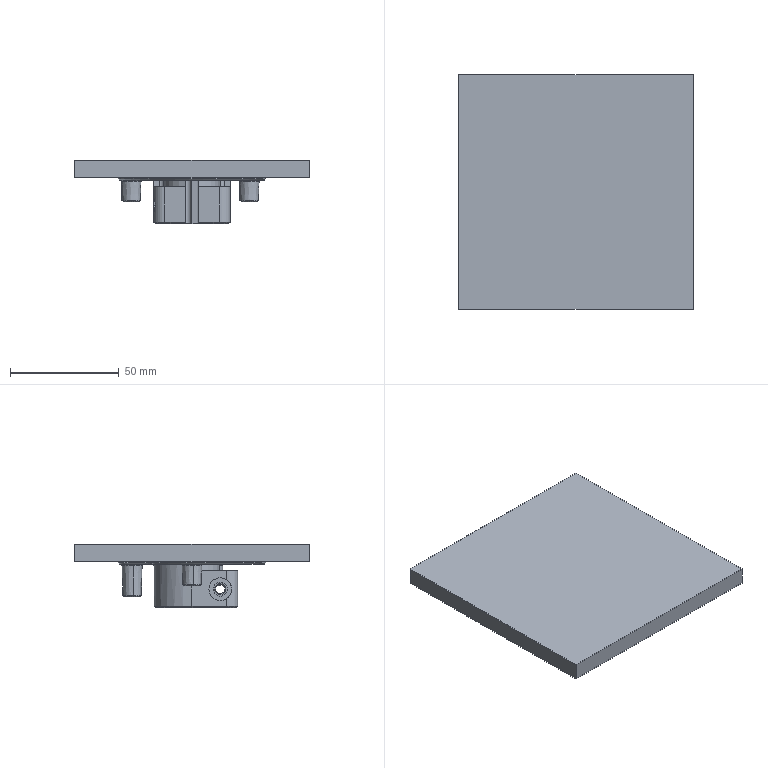NC program | NX | posted with a generic post | part box 108 x 108 x 29 mm
Lines 5648 to 6222 of 13118:
(ZLEVEL_PROFILE_COPY_COPY_COPY_1_COPY , TOOL : D4)
N11234 T15 M6
N11236 G54
N11238 G17 G0 G90 X-15.3 Y-3.944 S9500 M3
N11240 G43 Z30. H15
N11242 Z-0.4
N11244 G94 G1 X-14.797 Y-3.492 F1000.
N11246 G3 X-14.674 Y-3.112 R0.4
N11248 G2 X-14.866 Y-2. R15. F1500.
N11250 G1 X-16.015
N11252 G3 X-16.362 Y-2.2 R0.4
N11254 G1 Y-2.8
N11256 G0 X-15.3 Y-3.944 Z-0.8
N11258 G1 X-14.797 Y-3.492 F1000.
N11260 G3 X-14.674 Y-3.112 R0.4
N11262 G2 X-14.866 Y-2. R15. F1500.
N11264 G1 X-16.015
N11266 G3 X-16.362 Y-2.2 R0.4
N11268 G1 Y-2.8
N11270 G0 X-15.3 Y-3.944 Z-1.2
N11272 G1 X-14.797 Y-3.492 F1000.
N11274 G3 X-14.674 Y-3.112 R0.4
N11276 G2 X-14.866 Y-2. R15. F1500.
N11278 G1 X-16.015
N11280 G3 X-16.362 Y-2.2 R0.4
N11282 G1 Y-2.8
N11284 G0 X-15.3 Y-3.944 Z-1.6
N11286 G1 X-14.797 Y-3.492 F1000.
N11288 G3 X-14.674 Y-3.112 R0.4
N11290 G2 X-14.866 Y-2. R15. F1500.
N11292 G1 X-16.015
N11294 G3 X-16.362 Y-2.2 R0.4
N11296 G1 Y-2.8
N11298 G0 X-15.3 Y-3.944 Z-2.
N11300 G1 X-14.797 Y-3.492 F1000.
N11302 G3 X-14.674 Y-3.112 R0.4
N11304 G2 X-14.866 Y-2. R15. F1500.
N11306 G1 X-16.015
N11308 G3 X-16.362 Y-2.2 R0.4
N11310 G1 Y-2.8
N11312 G0 X-15.3 Y-3.944 Z-2.4
N11314 G1 X-14.797 Y-3.492 F1000.
N11316 G3 X-14.674 Y-3.112 R0.4
N11318 G2 X-14.866 Y-2. R15. F1500.
N11320 G1 X-16.015
N11322 G3 X-16.362 Y-2.2 R0.4
N11324 G1 Y-2.8
N11326 G0 X-15.3 Y-3.944 Z-2.8
N11328 G1 X-14.797 Y-3.492 F1000.
N11330 G3 X-14.674 Y-3.112 R0.4
N11332 G2 X-14.866 Y-2. R15. F1500.
N11334 G1 X-16.015
N11336 G3 X-16.362 Y-2.2 R0.4
N11338 G1 Y-2.8
N11340 G0 X-15.3 Y-3.944 Z-3.2
N11342 G1 X-14.797 Y-3.492 F1000.
N11344 G3 X-14.674 Y-3.112 R0.4
N11346 G2 X-14.866 Y-2. R15. F1500.
N11348 G1 X-16.015
N11350 G3 X-16.362 Y-2.2 R0.4
N11352 G1 Y-2.8
N11354 G0 X-15.3 Y-3.944 Z-3.6
N11356 G1 X-14.797 Y-3.492 F1000.
N11358 G3 X-14.674 Y-3.112 R0.4
N11360 G2 X-14.866 Y-2. R15. F1500.
N11362 G1 X-16.015
N11364 G3 X-16.362 Y-2.2 R0.4
N11366 G1 Y-2.8
N11368 G0 X-15.3 Y-3.944 Z-4.
N11370 G1 X-14.797 Y-3.492 F1000.
N11372 G3 X-14.674 Y-3.112 R0.4
N11374 G2 X-14.866 Y-2. R15. F1500.
N11376 G1 X-16.015
N11378 G3 X-16.362 Y-2.2 R0.4
N11380 G1 Y-2.8
N11382 G0 X-15.3 Y-3.944 Z-4.4
N11384 G1 X-14.797 Y-3.492 F1000.
N11386 G3 X-14.674 Y-3.112 R0.4
N11388 G2 X-14.866 Y-2. R15. F1500.
N11390 G1 X-16.015
N11392 G3 X-16.362 Y-2.2 R0.4
N11394 G1 Y-2.8
N11396 G0 X-15.3 Y-3.944 Z-4.8
N11398 G1 X-14.797 Y-3.492 F1000.
N11400 G3 X-14.674 Y-3.112 R0.4
N11402 G2 X-14.866 Y-2. R15. F1500.
N11404 G1 X-16.015
N11406 G3 X-16.362 Y-2.2 R0.4
N11408 G1 Y-2.8
N11410 G0 X-15.3 Y-3.944 Z-5.2
N11412 G1 X-14.797 Y-3.492 F1000.
N11414 G3 X-14.674 Y-3.112 R0.4
N11416 G2 X-14.866 Y-2. R15. F1500.
N11418 G1 X-16.015
N11420 G3 X-16.362 Y-2.2 R0.4
N11422 G1 Y-2.8
N11424 G0 X-15.3 Y-3.944 Z-5.6
N11426 G1 X-14.797 Y-3.492 F1000.
N11428 G3 X-14.674 Y-3.112 R0.4
N11430 G2 X-14.866 Y-2. R15. F1500.
N11432 G1 X-16.015
N11434 G3 X-16.362 Y-2.2 R0.4
N11436 G1 Y-2.8
N11438 G0 X-15.3 Y-3.944 Z-6.
N11440 G1 X-14.797 Y-3.492 F1000.
N11442 G3 X-14.674 Y-3.112 R0.4
N11444 G2 X-14.866 Y-2. R15. F1500.
N11446 G1 X-16.015
N11448 G3 X-16.362 Y-2.2 R0.4
N11450 G1 Y-2.8
N11452 G0 X-15.3 Y-3.944 Z-6.4
N11454 G1 X-14.797 Y-3.492 F1000.
N11456 G3 X-14.674 Y-3.112 R0.4
N11458 G2 X-14.866 Y-2. R15. F1500.
N11460 G1 X-16.015
N11462 G3 X-16.362 Y-2.2 R0.4
N11464 G1 Y-2.8
N11466 G0 X-15.3 Y-3.944 Z-6.8
N11468 G1 X-14.797 Y-3.492 F1000.
N11470 G3 X-14.674 Y-3.112 R0.4
N11472 G2 X-14.866 Y-2. R15. F1500.
N11474 G1 X-16.015
N11476 G3 X-16.362 Y-2.2 R0.4
N11478 G1 Y-2.8
N11480 G0 X-15.3 Y-3.944 Z-7.2
N11482 G1 X-14.797 Y-3.492 F1000.
N11484 G3 X-14.674 Y-3.112 R0.4
N11486 G2 X-14.866 Y-2. R15. F1500.
N11488 G1 X-16.015
N11490 G3 X-16.362 Y-2.2 R0.4
N11492 G1 Y-2.8
N11494 G0 X-15.3 Y-3.944 Z-7.6
N11496 G1 X-14.797 Y-3.492 F1000.
N11498 G3 X-14.674 Y-3.112 R0.4
N11500 G2 X-14.866 Y-2. R15. F1500.
N11502 G1 X-16.015
N11504 G3 X-16.362 Y-2.2 R0.4
N11506 G1 Y-2.8
N11508 G0 X-15.3 Y-3.944 Z-8.
N11510 G1 X-14.797 Y-3.492 F1000.
N11512 G3 X-14.674 Y-3.112 R0.4
N11514 G2 X-14.866 Y-2. R15. F1500.
N11516 G1 X-16.015
N11518 G3 X-16.362 Y-2.2 R0.4
N11520 G1 Y-2.8
N11522 G0 Z30.
N11524 X-15.855
N11526 Z-0.4
N11528 G1 Y-2.2 F1000.
N11530 G3 X-16.201 Y-2. R0.4
N11532 G1 X-17.5 F1500.
N11534 Y-3.299
N11536 G3 X-17.3 Y-3.645 R0.4
N11538 G1 X-16.7 Y-3.992
N11540 G0 X-15.855 Y-2.8 Z-0.8
N11542 G1 Y-2.2 F1000.
N11544 G3 X-16.201 Y-2. R0.4
N11546 G1 X-17.5 F1500.
N11548 Y-3.299
N11550 G3 X-17.3 Y-3.645 R0.4
N11552 G1 X-16.7 Y-3.992
N11554 G0 X-15.855 Y-2.8 Z-1.2
N11556 G1 Y-2.2 F1000.
N11558 G3 X-16.201 Y-2. R0.4
N11560 G1 X-17.5 F1500.
N11562 Y-3.299
N11564 G3 X-17.3 Y-3.645 R0.4
N11566 G1 X-16.7 Y-3.992
N11568 G0 X-15.855 Y-2.8 Z-1.6
N11570 G1 Y-2.2 F1000.
N11572 G3 X-16.201 Y-2. R0.4
N11574 G1 X-17.5 F1500.
N11576 Y-3.299
N11578 G3 X-17.3 Y-3.645 R0.4
N11580 G1 X-16.7 Y-3.992
N11582 G0 X-15.855 Y-2.8 Z-2.
N11584 G1 Y-2.2 F1000.
N11586 G3 X-16.201 Y-2. R0.4
N11588 G1 X-17.5 F1500.
N11590 Y-3.299
N11592 G3 X-17.3 Y-3.645 R0.4
N11594 G1 X-16.7 Y-3.992
N11596 G0 X-15.855 Y-2.8 Z-2.4
N11598 G1 Y-2.2 F1000.
N11600 G3 X-16.201 Y-2. R0.4
N11602 G1 X-17.5 F1500.
N11604 Y-3.299
N11606 G3 X-17.3 Y-3.645 R0.4
N11608 G1 X-16.7 Y-3.992
N11610 G0 X-15.855 Y-2.8 Z-2.8
N11612 G1 Y-2.2 F1000.
N11614 G3 X-16.201 Y-2. R0.4
N11616 G1 X-17.5 F1500.
N11618 Y-3.299
N11620 G3 X-17.3 Y-3.645 R0.4
N11622 G1 X-16.7 Y-3.992
N11624 G0 X-15.855 Y-2.8 Z-3.2
N11626 G1 Y-2.2 F1000.
N11628 G3 X-16.201 Y-2. R0.4
N11630 G1 X-17.5 F1500.
N11632 Y-3.299
N11634 G3 X-17.3 Y-3.645 R0.4
N11636 G1 X-16.7 Y-3.992
N11638 G0 X-15.855 Y-2.8 Z-3.6
N11640 G1 Y-2.2 F1000.
N11642 G3 X-16.201 Y-2. R0.4
N11644 G1 X-17.5 F1500.
N11646 Y-3.299
N11648 G3 X-17.3 Y-3.645 R0.4
N11650 G1 X-16.7 Y-3.992
N11652 G0 X-15.855 Y-2.8 Z-4.
N11654 G1 Y-2.2 F1000.
N11656 G3 X-16.201 Y-2. R0.4
N11658 G1 X-17.5 F1500.
N11660 Y-3.299
N11662 G3 X-17.3 Y-3.645 R0.4
N11664 G1 X-16.7 Y-3.992
N11666 G0 X-15.855 Y-2.8 Z-4.4
N11668 G1 Y-2.2 F1000.
N11670 G3 X-16.201 Y-2. R0.4
N11672 G1 X-17.5 F1500.
N11674 Y-3.299
N11676 G3 X-17.3 Y-3.645 R0.4
N11678 G1 X-16.7 Y-3.992
N11680 G0 X-15.855 Y-2.8 Z-4.8
N11682 G1 Y-2.2 F1000.
N11684 G3 X-16.201 Y-2. R0.4
N11686 G1 X-17.5 F1500.
N11688 Y-3.299
N11690 G3 X-17.3 Y-3.645 R0.4
N11692 G1 X-16.7 Y-3.992
N11694 G0 X-15.855 Y-2.8 Z-5.2
N11696 G1 Y-2.2 F1000.
N11698 G3 X-16.201 Y-2. R0.4
N11700 G1 X-17.5 F1500.
N11702 Y-3.299
N11704 G3 X-17.3 Y-3.645 R0.4
N11706 G1 X-16.7 Y-3.992
N11708 G0 X-15.855 Y-2.8 Z-5.6
N11710 G1 Y-2.2 F1000.
N11712 G3 X-16.201 Y-2. R0.4
N11714 G1 X-17.5 F1500.
N11716 Y-3.299
N11718 G3 X-17.3 Y-3.646 R0.4
N11720 G1 X-16.7 Y-3.992
N11722 G0 X-15.855 Y-2.8 Z-6.
N11724 G1 Y-2.2 F1000.
N11726 G3 X-16.201 Y-2. R0.4
N11728 G1 X-17.5 F1500.
N11730 Y-3.299
N11732 G3 X-17.3 Y-3.645 R0.4
N11734 G1 X-16.7 Y-3.992
N11736 G0 X-15.854 Y-2.8 Z-6.4
N11738 G1 Y-2.2 F1000.
N11740 G3 X-16.201 Y-2. R0.4
N11742 G1 X-17.5 F1500.
N11744 Y-3.3
N11746 G3 X-17.3 Y-3.646 R0.4
N11748 G1 X-16.7 Y-3.992
N11750 G0 X-15.855 Y-2.8 Z-6.8
N11752 G1 Y-2.2 F1000.
N11754 G3 X-16.201 Y-2. R0.4
N11756 G1 X-17.5 F1500.
N11758 Y-3.299
N11760 G3 X-17.3 Y-3.645 R0.4
N11762 G1 X-16.7 Y-3.992
N11764 G0 X-15.854 Y-2.8 Z-7.2
N11766 G1 Y-2.2 F1000.
N11768 G3 X-16.201 Y-2. R0.4
N11770 G1 X-17.5 F1500.
N11772 Y-3.3
N11774 G3 X-17.3 Y-3.646 R0.4
N11776 G1 X-16.7 Y-3.993
N11778 G0 X-15.855 Y-2.8 Z-7.6
N11780 G1 Y-2.2 F1000.
N11782 G3 X-16.201 Y-2. R0.4
N11784 G1 X-17.5 F1500.
N11786 Y-3.299
N11788 G3 X-17.3 Y-3.645 R0.4
N11790 G1 X-16.7 Y-3.992
N11792 G0 X-15.854 Y-2.8 Z-8.
N11794 G1 Y-2.2 F1000.
N11796 G3 X-16.201 Y-2. R0.4
N11798 G1 X-17.5 F1500.
N11800 Y-3.301
N11802 G3 X-17.3 Y-3.648 R0.4
N11804 G1 X-16.7 Y-3.994
N11806 G0 Z30.
N11808 X16.7 Y-3.992
N11810 Z-0.4
N11812 G1 X17.3 Y-3.645 F1000.
N11814 G3 X17.5 Y-3.299 R0.4
N11816 G1 Y-2. F1500.
N11818 X16.201
N11820 G3 X15.855 Y-2.2 R0.4
N11822 G1 Y-2.8
N11824 G0 X16.7 Y-3.992 Z-0.8
N11826 G1 X17.3 Y-3.645 F1000.
N11828 G3 X17.5 Y-3.299 R0.4
N11830 G1 Y-2. F1500.
N11832 X16.201
N11834 G3 X15.855 Y-2.2 R0.4
N11836 G1 Y-2.8
N11838 G0 X16.7 Y-3.992 Z-1.2
N11840 G1 X17.3 Y-3.645 F1000.
N11842 G3 X17.5 Y-3.299 R0.4
N11844 G1 Y-2. F1500.
N11846 X16.201
N11848 G3 X15.855 Y-2.2 R0.4
N11850 G1 Y-2.8
N11852 G0 X16.7 Y-3.992 Z-1.6
N11854 G1 X17.3 Y-3.645 F1000.
N11856 G3 X17.5 Y-3.299 R0.4
N11858 G1 Y-2. F1500.
N11860 X16.201
N11862 G3 X15.855 Y-2.2 R0.4
N11864 G1 Y-2.8
N11866 G0 X16.7 Y-3.992 Z-2.
N11868 G1 X17.3 Y-3.645 F1000.
N11870 G3 X17.5 Y-3.299 R0.4
N11872 G1 Y-2. F1500.
N11874 X16.201
N11876 G3 X15.855 Y-2.2 R0.4
N11878 G1 Y-2.8
N11880 G0 X16.7 Y-3.992 Z-2.4
N11882 G1 X17.3 Y-3.645 F1000.
N11884 G3 X17.5 Y-3.299 R0.4
N11886 G1 Y-2. F1500.
N11888 X16.201
N11890 G3 X15.855 Y-2.2 R0.4
N11892 G1 Y-2.8
N11894 G0 X16.7 Y-3.992 Z-2.8
N11896 G1 X17.3 Y-3.645 F1000.
N11898 G3 X17.5 Y-3.299 R0.4
N11900 G1 Y-2. F1500.
N11902 X16.201
N11904 G3 X15.855 Y-2.2 R0.4
N11906 G1 Y-2.8
N11908 G0 X16.7 Y-3.992 Z-3.2
N11910 G1 X17.3 Y-3.645 F1000.
N11912 G3 X17.5 Y-3.299 R0.4
N11914 G1 Y-2. F1500.
N11916 X16.201
N11918 G3 X15.855 Y-2.2 R0.4
N11920 G1 Y-2.8
N11922 G0 X16.7 Y-3.992 Z-3.6
N11924 G1 X17.3 Y-3.645 F1000.
N11926 G3 X17.5 Y-3.299 R0.4
N11928 G1 Y-2. F1500.
N11930 X16.201
N11932 G3 X15.855 Y-2.2 R0.4
N11934 G1 Y-2.8
N11936 G0 X16.7 Y-3.992 Z-4.
N11938 G1 X17.3 Y-3.645 F1000.
N11940 G3 X17.5 Y-3.299 R0.4
N11942 G1 Y-2. F1500.
N11944 X16.201
N11946 G3 X15.855 Y-2.2 R0.4
N11948 G1 Y-2.8
N11950 G0 X16.7 Y-3.992 Z-4.4
N11952 G1 X17.3 Y-3.645 F1000.
N11954 G3 X17.5 Y-3.299 R0.4
N11956 G1 Y-2. F1500.
N11958 X16.201
N11960 G3 X15.855 Y-2.2 R0.4
N11962 G1 Y-2.8
N11964 G0 X16.7 Y-3.992 Z-4.8
N11966 G1 X17.3 Y-3.645 F1000.
N11968 G3 X17.5 Y-3.299 R0.4
N11970 G1 Y-2. F1500.
N11972 X16.201
N11974 G3 X15.855 Y-2.2 R0.4
N11976 G1 Y-2.8
N11978 G0 X16.7 Y-3.992 Z-5.2
N11980 G1 X17.3 Y-3.645 F1000.
N11982 G3 X17.5 Y-3.299 R0.4
N11984 G1 Y-2. F1500.
N11986 X16.201
N11988 G3 X15.855 Y-2.2 R0.4
N11990 G1 Y-2.8
N11992 G0 X16.7 Y-3.992 Z-5.6
N11994 G1 X17.3 Y-3.646 F1000.
N11996 G3 X17.5 Y-3.299 R0.4
N11998 G1 Y-2. F1500.
N12000 X16.201
N12002 G3 X15.855 Y-2.2 R0.4
N12004 G1 Y-2.8
N12006 G0 X16.7 Y-3.992 Z-6.
N12008 G1 X17.3 Y-3.645 F1000.
N12010 G3 X17.5 Y-3.299 R0.4
N12012 G1 Y-2. F1500.
N12014 X16.201
N12016 G3 X15.855 Y-2.2 R0.4
N12018 G1 Y-2.8
N12020 G0 X16.7 Y-3.992 Z-6.4
N12022 G1 X17.3 Y-3.646 F1000.
N12024 G3 X17.5 Y-3.3 R0.4
N12026 G1 Y-2. F1500.
N12028 X16.201
N12030 G3 X15.854 Y-2.2 R0.4
N12032 G1 Y-2.8
N12034 G0 X16.7 Y-3.992 Z-6.8
N12036 G1 X17.3 Y-3.645 F1000.
N12038 G3 X17.5 Y-3.299 R0.4
N12040 G1 Y-2. F1500.
N12042 X16.201
N12044 G3 X15.855 Y-2.2 R0.4
N12046 G1 Y-2.8
N12048 G0 X16.7 Y-3.993 Z-7.2
N12050 G1 X17.3 Y-3.646 F1000.
N12052 G3 X17.5 Y-3.3 R0.4
N12054 G1 Y-2. F1500.
N12056 X16.201
N12058 G3 X15.854 Y-2.2 R0.4
N12060 G1 Y-2.8
N12062 G0 X16.7 Y-3.992 Z-7.6
N12064 G1 X17.3 Y-3.645 F1000.
N12066 G3 X17.5 Y-3.299 R0.4
N12068 G1 Y-2. F1500.
N12070 X16.201
N12072 G3 X15.855 Y-2.2 R0.4
N12074 G1 Y-2.8
N12076 G0 X16.7 Y-3.994 Z-8.
N12078 G1 X17.3 Y-3.648 F1000.
N12080 G3 X17.5 Y-3.301 R0.4
N12082 G1 Y-2. F1500.
N12084 X16.201
N12086 G3 X15.854 Y-2.2 R0.4
N12088 G1 Y-2.8
N12090 G0 Z30.
N12092 X16.362
N12094 Z-0.4
N12096 G1 Y-2.2 F1000.
N12098 G3 X16.015 Y-2. R0.4
N12100 G1 X14.866 F1500.
N12102 G2 X14.674 Y-3.112 R15.
N12104 G3 X14.797 Y-3.492 R0.4
N12106 G1 X15.3 Y-3.944
N12108 G0 X16.362 Y-2.8 Z-0.8
N12110 G1 Y-2.2 F1000.
N12112 G3 X16.015 Y-2. R0.4
N12114 G1 X14.866 F1500.
N12116 G2 X14.674 Y-3.112 R15.
N12118 G3 X14.797 Y-3.492 R0.4
N12120 G1 X15.3 Y-3.944
N12122 G0 X16.362 Y-2.8 Z-1.2
N12124 G1 Y-2.2 F1000.
N12126 G3 X16.015 Y-2. R0.4
N12128 G1 X14.866 F1500.
N12130 G2 X14.674 Y-3.112 R15.
N12132 G3 X14.797 Y-3.492 R0.4
N12134 G1 X15.3 Y-3.944
N12136 G0 X16.362 Y-2.8 Z-1.6
N12138 G1 Y-2.2 F1000.
N12140 G3 X16.015 Y-2. R0.4
N12142 G1 X14.866 F1500.
N12144 G2 X14.674 Y-3.112 R15.
N12146 G3 X14.797 Y-3.492 R0.4
N12148 G1 X15.3 Y-3.944
N12150 G0 X16.362 Y-2.8 Z-2.
N12152 G1 Y-2.2 F1000.
N12154 G3 X16.015 Y-2. R0.4
N12156 G1 X14.866 F1500.
N12158 G2 X14.674 Y-3.112 R15.
N12160 G3 X14.797 Y-3.492 R0.4
N12162 G1 X15.3 Y-3.944
N12164 G0 X16.362 Y-2.8 Z-2.4
N12166 G1 Y-2.2 F1000.
N12168 G3 X16.015 Y-2. R0.4
N12170 G1 X14.866 F1500.
N12172 G2 X14.674 Y-3.112 R15.
N12174 G3 X14.797 Y-3.492 R0.4
N12176 G1 X15.3 Y-3.944
N12178 G0 X16.362 Y-2.8 Z-2.8
N12180 G1 Y-2.2 F1000.
N12182 G3 X16.015 Y-2. R0.4
N12184 G1 X14.866 F1500.
N12186 G2 X14.674 Y-3.112 R15.
N12188 G3 X14.797 Y-3.492 R0.4
N12190 G1 X15.3 Y-3.944
N12192 G0 X16.362 Y-2.8 Z-3.2
N12194 G1 Y-2.2 F1000.
N12196 G3 X16.015 Y-2. R0.4
N12198 G1 X14.866 F1500.
N12200 G2 X14.674 Y-3.112 R15.
N12202 G3 X14.797 Y-3.492 R0.4
N12204 G1 X15.3 Y-3.944
N12206 G0 X16.362 Y-2.8 Z-3.6
N12208 G1 Y-2.2 F1000.
N12210 G3 X16.015 Y-2. R0.4
N12212 G1 X14.866 F1500.
N12214 G2 X14.674 Y-3.112 R15.
N12216 G3 X14.797 Y-3.492 R0.4
N12218 G1 X15.3 Y-3.944
N12220 G0 X16.362 Y-2.8 Z-4.
N12222 G1 Y-2.2 F1000.
N12224 G3 X16.015 Y-2. R0.4
N12226 G1 X14.866 F1500.
N12228 G2 X14.674 Y-3.112 R15.
N12230 G3 X14.797 Y-3.492 R0.4
N12232 G1 X15.3 Y-3.944
N12234 G0 X16.362 Y-2.8 Z-4.4
N12236 G1 Y-2.2 F1000.
N12238 G3 X16.015 Y-2. R0.4
N12240 G1 X14.866 F1500.
N12242 G2 X14.674 Y-3.112 R15.
N12244 G3 X14.797 Y-3.492 R0.4
N12246 G1 X15.3 Y-3.944
N12248 G0 X16.362 Y-2.8 Z-4.8
N12250 G1 Y-2.2 F1000.
N12252 G3 X16.015 Y-2. R0.4
N12254 G1 X14.866 F1500.
N12256 G2 X14.674 Y-3.112 R15.
N12258 G3 X14.797 Y-3.492 R0.4
N12260 G1 X15.3 Y-3.944
N12262 G0 X16.362 Y-2.8 Z-5.2
N12264 G1 Y-2.2 F1000.
N12266 G3 X16.015 Y-2. R0.4
N12268 G1 X14.866 F1500.
N12270 G2 X14.674 Y-3.112 R15.
N12272 G3 X14.797 Y-3.492 R0.4
N12274 G1 X15.3 Y-3.944
N12276 G0 X16.362 Y-2.8 Z-5.6
N12278 G1 Y-2.2 F1000.
N12280 G3 X16.015 Y-2. R0.4
N12282 G1 X14.866 F1500.
N12284 G2 X14.674 Y-3.112 R15.
N12286 G3 X14.797 Y-3.492 R0.4
N12288 G1 X15.3 Y-3.944
N12290 G0 X16.362 Y-2.8 Z-6.
N12292 G1 Y-2.2 F1000.
N12294 G3 X16.015 Y-2. R0.4
N12296 G1 X14.866 F1500.
N12298 G2 X14.674 Y-3.112 R15.
N12300 G3 X14.797 Y-3.492 R0.4
N12302 G1 X15.3 Y-3.944
N12304 G0 X16.362 Y-2.8 Z-6.4
N12306 G1 Y-2.2 F1000.
N12308 G3 X16.015 Y-2. R0.4
N12310 G1 X14.866 F1500.
N12312 G2 X14.674 Y-3.112 R15.
N12314 G3 X14.797 Y-3.492 R0.4
N12316 G1 X15.3 Y-3.944
N12318 G0 X16.362 Y-2.8 Z-6.8
N12320 G1 Y-2.2 F1000.
N12322 G3 X16.015 Y-2. R0.4
N12324 G1 X14.866 F1500.
N12326 G2 X14.674 Y-3.112 R15.
N12328 G3 X14.797 Y-3.492 R0.4
N12330 G1 X15.3 Y-3.944
N12332 G0 X16.362 Y-2.8 Z-7.2
N12334 G1 Y-2.2 F1000.
N12336 G3 X16.015 Y-2. R0.4
N12338 G1 X14.866 F1500.
N12340 G2 X14.674 Y-3.112 R15.
N12342 G3 X14.797 Y-3.492 R0.4
N12344 G1 X15.3 Y-3.944
N12346 G0 X16.362 Y-2.8 Z-7.6
N12348 G1 Y-2.2 F1000.
N12350 G3 X16.015 Y-2. R0.4
N12352 G1 X14.866 F1500.
N12354 G2 X14.674 Y-3.112 R15.
N12356 G3 X14.797 Y-3.492 R0.4
N12358 G1 X15.3 Y-3.944
N12360 G0 X16.362 Y-2.8 Z-8.
N12362 G1 Y-2.2 F1000.
N12364 G3 X16.015 Y-2. R0.4
N12366 G1 X14.866 F1500.
N12368 G2 X14.674 Y-3.112 R15.
N12370 G3 X14.797 Y-3.492 R0.4
N12372 G1 X15.3 Y-3.944
N12374 G0 Z30.
N12376 M5